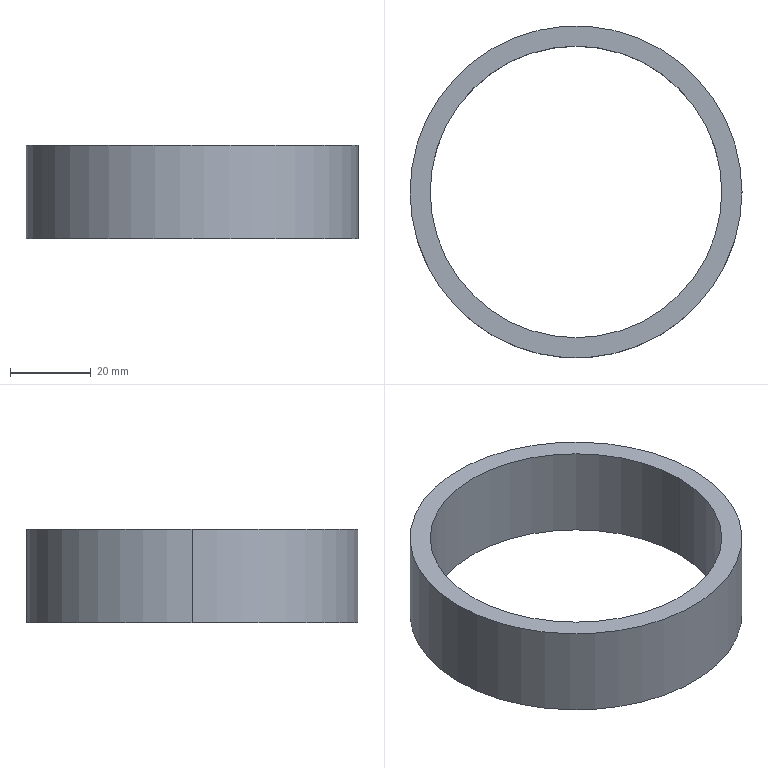Part | STEP file | Spindle Inner Spacer | 1 solid | 6 faces | box 82 x 82 x 23 mm | volume 27819 mm3 | cylinder 4 | plane 2 | commonest cylinder face diameters 72 x2 82 x2
STEP:
#1=CARTESIAN_POINT('',(-41.,0.,23.));
#2=VERTEX_POINT('',#1);
#3=CARTESIAN_POINT('',(41.,0.,23.));
#4=VERTEX_POINT('',#3);
#5=CARTESIAN_POINT('',(0.,0.,23.));
#6=DIRECTION('',(0.,0.,-1.));
#7=DIRECTION('',(-1.,0.,0.));
#8=AXIS2_PLACEMENT_3D('',#5,#6,#7);
#9=CIRCLE('',#8,41.);
#10=EDGE_CURVE('',#2,#4,#9,.T.);
#11=ORIENTED_EDGE('',*,*,#10,.T.);
#12=CARTESIAN_POINT('',(41.,0.,0.));
#13=VERTEX_POINT('',#12);
#14=CARTESIAN_POINT('',(41.,0.,23.));
#15=DIRECTION('',(0.,0.,-1.));
#16=VECTOR('',#15,1000.);
#17=LINE('',#14,#16);
#18=EDGE_CURVE('',#4,#13,#17,.T.);
#19=ORIENTED_EDGE('',*,*,#18,.T.);
#20=CARTESIAN_POINT('',(-41.,0.,0.));
#21=VERTEX_POINT('',#20);
#22=CARTESIAN_POINT('',(0.,0.,0.));
#23=DIRECTION('',(0.,0.,1.));
#24=DIRECTION('',(-1.,0.,0.));
#25=AXIS2_PLACEMENT_3D('',#22,#23,#24);
#26=CIRCLE('',#25,41.);
#27=EDGE_CURVE('',#13,#21,#26,.T.);
#28=ORIENTED_EDGE('',*,*,#27,.T.);
#29=CARTESIAN_POINT('',(-41.,0.,23.));
#30=DIRECTION('',(0.,0.,-1.));
#31=VECTOR('',#30,1000.);
#32=LINE('',#29,#31);
#33=EDGE_CURVE('',#2,#21,#32,.T.);
#34=ORIENTED_EDGE('',*,*,#33,.F.);
#35=EDGE_LOOP('',(#11,#19,#28,#34));
#36=FACE_OUTER_BOUND('',#35,.T.);
#37=CARTESIAN_POINT('',(0.,0.,23.));
#38=DIRECTION('',(0.,0.,-1.));
#39=DIRECTION('',(-1.,0.,0.));
#40=AXIS2_PLACEMENT_3D('',#37,#38,#39);
#41=CYLINDRICAL_SURFACE('',#40,41.);
#42=ADVANCED_FACE('',(#36),#41,.T.);
#43=CARTESIAN_POINT('',(36.,0.,23.));
#44=VERTEX_POINT('',#43);
#45=CARTESIAN_POINT('',(-36.,0.,23.));
#46=VERTEX_POINT('',#45);
#47=CARTESIAN_POINT('',(0.,0.,23.));
#48=DIRECTION('',(0.,0.,-1.));
#49=DIRECTION('',(-1.,0.,0.));
#50=AXIS2_PLACEMENT_3D('',#47,#48,#49);
#51=CIRCLE('',#50,36.);
#52=EDGE_CURVE('',#44,#46,#51,.T.);
#53=ORIENTED_EDGE('',*,*,#52,.F.);
#54=CARTESIAN_POINT('',(36.,0.,0.));
#55=VERTEX_POINT('',#54);
#56=CARTESIAN_POINT('',(36.,0.,23.));
#57=DIRECTION('',(0.,0.,-1.));
#58=VECTOR('',#57,1000.);
#59=LINE('',#56,#58);
#60=EDGE_CURVE('',#44,#55,#59,.T.);
#61=ORIENTED_EDGE('',*,*,#60,.T.);
#62=CARTESIAN_POINT('',(-36.,0.,0.));
#63=VERTEX_POINT('',#62);
#64=CARTESIAN_POINT('',(0.,0.,0.));
#65=DIRECTION('',(0.,0.,-1.));
#66=DIRECTION('',(-1.,0.,0.));
#67=AXIS2_PLACEMENT_3D('',#64,#65,#66);
#68=CIRCLE('',#67,36.);
#69=EDGE_CURVE('',#55,#63,#68,.T.);
#70=ORIENTED_EDGE('',*,*,#69,.T.);
#71=CARTESIAN_POINT('',(-36.,0.,23.));
#72=DIRECTION('',(0.,0.,-1.));
#73=VECTOR('',#72,1000.);
#74=LINE('',#71,#73);
#75=EDGE_CURVE('',#46,#63,#74,.T.);
#76=ORIENTED_EDGE('',*,*,#75,.F.);
#77=EDGE_LOOP('',(#53,#61,#70,#76));
#78=FACE_OUTER_BOUND('',#77,.T.);
#79=CARTESIAN_POINT('',(0.,0.,23.));
#80=DIRECTION('',(0.,0.,-1.));
#81=DIRECTION('',(-1.,0.,0.));
#82=AXIS2_PLACEMENT_3D('',#79,#80,#81);
#83=CYLINDRICAL_SURFACE('',#82,36.);
#84=ADVANCED_FACE('',(#78),#83,.F.);
#85=ORIENTED_EDGE('',*,*,#18,.F.);
#86=CARTESIAN_POINT('',(0.,0.,23.));
#87=DIRECTION('',(0.,0.,-1.));
#88=DIRECTION('',(-1.,0.,0.));
#89=AXIS2_PLACEMENT_3D('',#86,#87,#88);
#90=CIRCLE('',#89,41.);
#91=EDGE_CURVE('',#4,#2,#90,.T.);
#92=ORIENTED_EDGE('',*,*,#91,.T.);
#93=ORIENTED_EDGE('',*,*,#33,.T.);
#94=CARTESIAN_POINT('',(0.,0.,0.));
#95=DIRECTION('',(0.,0.,1.));
#96=DIRECTION('',(-1.,0.,0.));
#97=AXIS2_PLACEMENT_3D('',#94,#95,#96);
#98=CIRCLE('',#97,41.);
#99=EDGE_CURVE('',#21,#13,#98,.T.);
#100=ORIENTED_EDGE('',*,*,#99,.T.);
#101=EDGE_LOOP('',(#85,#92,#93,#100));
#102=FACE_OUTER_BOUND('',#101,.T.);
#103=CARTESIAN_POINT('',(0.,0.,23.));
#104=DIRECTION('',(0.,0.,-1.));
#105=DIRECTION('',(-1.,0.,0.));
#106=AXIS2_PLACEMENT_3D('',#103,#104,#105);
#107=CYLINDRICAL_SURFACE('',#106,41.);
#108=ADVANCED_FACE('',(#102),#107,.T.);
#109=CARTESIAN_POINT('',(0.,0.,0.));
#110=DIRECTION('',(0.,0.,-1.));
#111=DIRECTION('',(-1.,0.,0.));
#112=AXIS2_PLACEMENT_3D('',#109,#110,#111);
#113=CIRCLE('',#112,36.);
#114=EDGE_CURVE('',#63,#55,#113,.T.);
#115=ORIENTED_EDGE('',*,*,#114,.F.);
#116=ORIENTED_EDGE('',*,*,#69,.F.);
#117=EDGE_LOOP('',(#115,#116));
#118=FACE_BOUND('',#117,.T.);
#119=ORIENTED_EDGE('',*,*,#99,.F.);
#120=ORIENTED_EDGE('',*,*,#27,.F.);
#121=EDGE_LOOP('',(#119,#120));
#122=FACE_OUTER_BOUND('',#121,.T.);
#123=CARTESIAN_POINT('',(0.,0.,0.));
#124=DIRECTION('',(0.,0.,1.));
#125=DIRECTION('',(1.,0.,0.));
#126=AXIS2_PLACEMENT_3D('',#123,#124,#125);
#127=PLANE('',#126);
#128=ADVANCED_FACE('',(#118,#122),#127,.F.);
#129=CARTESIAN_POINT('',(0.,0.,23.));
#130=DIRECTION('',(0.,0.,-1.));
#131=DIRECTION('',(-1.,0.,0.));
#132=AXIS2_PLACEMENT_3D('',#129,#130,#131);
#133=CIRCLE('',#132,36.);
#134=EDGE_CURVE('',#46,#44,#133,.T.);
#135=ORIENTED_EDGE('',*,*,#134,.T.);
#136=ORIENTED_EDGE('',*,*,#52,.T.);
#137=EDGE_LOOP('',(#135,#136));
#138=FACE_BOUND('',#137,.T.);
#139=ORIENTED_EDGE('',*,*,#10,.F.);
#140=ORIENTED_EDGE('',*,*,#91,.F.);
#141=EDGE_LOOP('',(#139,#140));
#142=FACE_OUTER_BOUND('',#141,.T.);
#143=CARTESIAN_POINT('',(0.,0.,23.));
#144=DIRECTION('',(0.,0.,1.));
#145=DIRECTION('',(1.,0.,0.));
#146=AXIS2_PLACEMENT_3D('',#143,#144,#145);
#147=PLANE('',#146);
#148=ADVANCED_FACE('',(#138,#142),#147,.T.);
#149=ORIENTED_EDGE('',*,*,#60,.F.);
#150=ORIENTED_EDGE('',*,*,#134,.F.);
#151=ORIENTED_EDGE('',*,*,#75,.T.);
#152=ORIENTED_EDGE('',*,*,#114,.T.);
#153=EDGE_LOOP('',(#149,#150,#151,#152));
#154=FACE_OUTER_BOUND('',#153,.T.);
#155=CARTESIAN_POINT('',(0.,0.,23.));
#156=DIRECTION('',(0.,0.,-1.));
#157=DIRECTION('',(-1.,0.,0.));
#158=AXIS2_PLACEMENT_3D('',#155,#156,#157);
#159=CYLINDRICAL_SURFACE('',#158,36.);
#160=ADVANCED_FACE('',(#154),#159,.F.);
#161=CLOSED_SHELL('',(#42,#84,#108,#128,#148,#160));
#162=MANIFOLD_SOLID_BREP('',#161);
#163=CARTESIAN_POINT('',(0.,0.,0.));
#164=DIRECTION('',(0.,0.,1.));
#165=DIRECTION('',(1.,0.,0.));
#166=AXIS2_PLACEMENT_3D('',#163,#164,#165);
#167=(LENGTH_UNIT()NAMED_UNIT(*)SI_UNIT(.MILLI.,.METRE.));
#168=UNCERTAINTY_MEASURE_WITH_UNIT(LENGTH_MEASURE(0.00001),#167,'','');
#169=(NAMED_UNIT(*)PLANE_ANGLE_UNIT()SI_UNIT($,.RADIAN.));
#170=(NAMED_UNIT(*)SI_UNIT($,.STERADIAN.)SOLID_ANGLE_UNIT());
#171=(GEOMETRIC_REPRESENTATION_CONTEXT(3)GLOBAL_UNCERTAINTY_ASSIGNED_CONTEXT((#168))GLOBAL_UNIT_ASSIGNED_CONTEXT((#167,#169,#170))REPRESENTATION_CONTEXT('',''));
#172=ADVANCED_BREP_SHAPE_REPRESENTATION('',(#162,#166),#171);